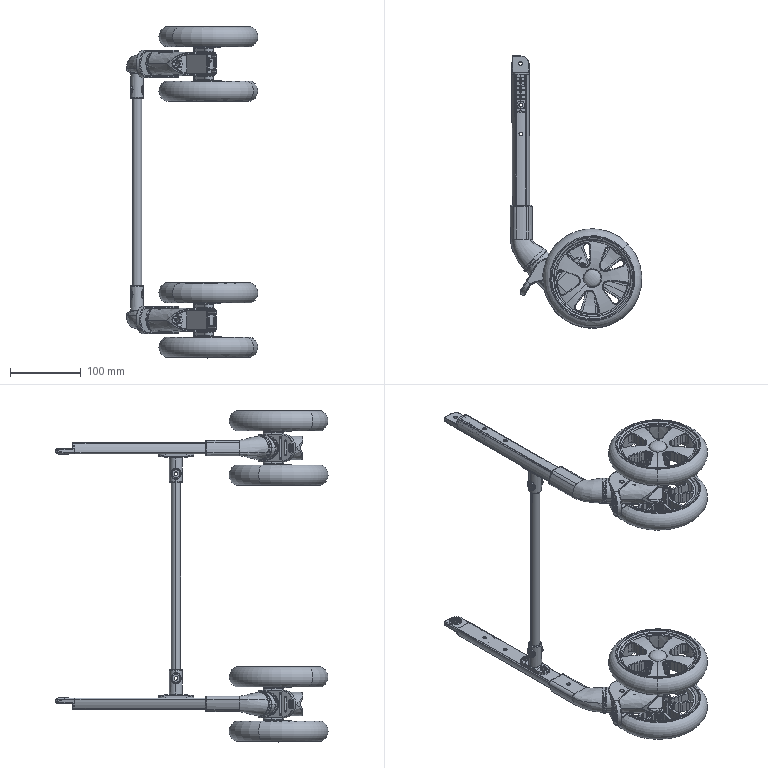Part | SolidWorks | 35 solids | 5475 faces | volume 1026914 mm3 | spline 2294 | cylinder 1516 | plane 1064 | torus 387 | cone 116 | sphere 98 | commonest cylinder face diameters 1 x226 0.6 x222 2 x84 4 x84 10 x74 7 x56